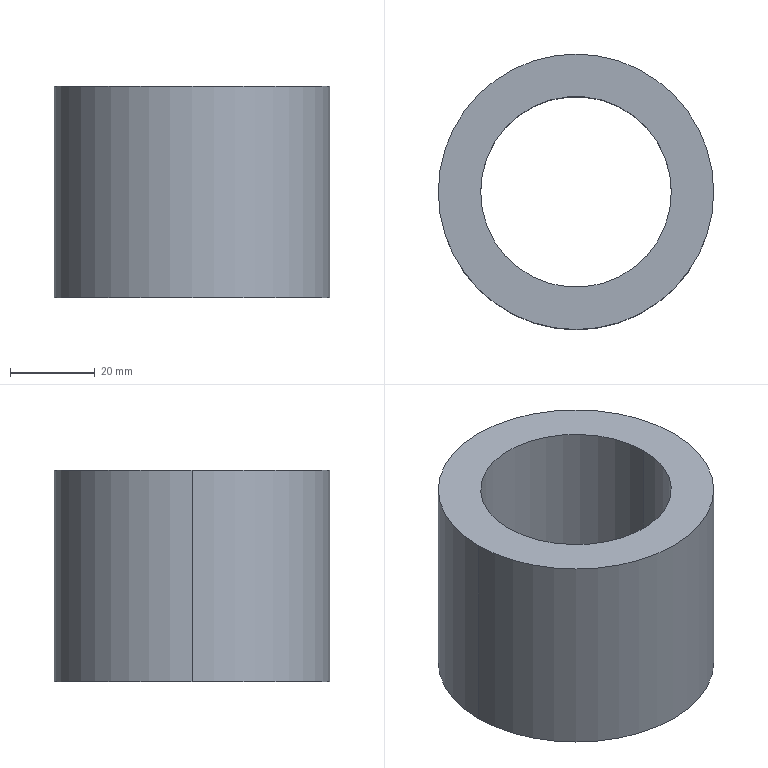Part | SolidWorks | features Extrusion 1 | 1 solid | 6 faces | box 65 x 65 x 50 mm | volume 86394 mm3 | cylinder 4 | plane 2 | commonest cylinder face diameters 45 x2 65 x2
STEP:
#1=CARTESIAN_POINT('',(-22.5,0.,50.));
#2=VERTEX_POINT('',#1);
#3=CARTESIAN_POINT('',(22.5,0.,50.));
#4=VERTEX_POINT('',#3);
#5=CARTESIAN_POINT('',(0.,0.,50.));
#6=DIRECTION('',(0.,0.,1.));
#7=DIRECTION('',(1.,0.,0.));
#8=AXIS2_PLACEMENT_3D('',#5,#6,#7);
#9=CIRCLE('',#8,22.5);
#10=EDGE_CURVE('',#2,#4,#9,.T.);
#11=ORIENTED_EDGE('',*,*,#10,.T.);
#12=CARTESIAN_POINT('',(22.5,0.,0.));
#13=VERTEX_POINT('',#12);
#14=CARTESIAN_POINT('',(22.5,0.,50.));
#15=DIRECTION('',(0.,0.,-1.));
#16=VECTOR('',#15,1000.);
#17=LINE('',#14,#16);
#18=EDGE_CURVE('',#4,#13,#17,.T.);
#19=ORIENTED_EDGE('',*,*,#18,.T.);
#20=CARTESIAN_POINT('',(-22.5,0.,0.));
#21=VERTEX_POINT('',#20);
#22=CARTESIAN_POINT('',(0.,0.,0.));
#23=DIRECTION('',(0.,0.,1.));
#24=DIRECTION('',(1.,0.,0.));
#25=AXIS2_PLACEMENT_3D('',#22,#23,#24);
#26=CIRCLE('',#25,22.5);
#27=EDGE_CURVE('',#21,#13,#26,.T.);
#28=ORIENTED_EDGE('',*,*,#27,.F.);
#29=CARTESIAN_POINT('',(-22.5,0.,50.));
#30=DIRECTION('',(0.,0.,-1.));
#31=VECTOR('',#30,1000.);
#32=LINE('',#29,#31);
#33=EDGE_CURVE('',#2,#21,#32,.T.);
#34=ORIENTED_EDGE('',*,*,#33,.F.);
#35=EDGE_LOOP('',(#11,#19,#28,#34));
#36=FACE_OUTER_BOUND('',#35,.T.);
#37=CARTESIAN_POINT('',(0.,0.,50.));
#38=DIRECTION('',(0.,0.,-1.));
#39=DIRECTION('',(-1.,0.,0.));
#40=AXIS2_PLACEMENT_3D('',#37,#38,#39);
#41=CYLINDRICAL_SURFACE('',#40,22.5);
#42=ADVANCED_FACE('',(#36),#41,.F.);
#43=CARTESIAN_POINT('',(32.5,0.,50.));
#44=VERTEX_POINT('',#43);
#45=CARTESIAN_POINT('',(-32.5,0.,50.));
#46=VERTEX_POINT('',#45);
#47=CARTESIAN_POINT('',(0.,0.,50.));
#48=DIRECTION('',(0.,0.,1.));
#49=DIRECTION('',(1.,0.,0.));
#50=AXIS2_PLACEMENT_3D('',#47,#48,#49);
#51=CIRCLE('',#50,32.5);
#52=EDGE_CURVE('',#44,#46,#51,.T.);
#53=ORIENTED_EDGE('',*,*,#52,.F.);
#54=CARTESIAN_POINT('',(32.5,0.,0.));
#55=VERTEX_POINT('',#54);
#56=CARTESIAN_POINT('',(32.5,0.,50.));
#57=DIRECTION('',(0.,0.,-1.));
#58=VECTOR('',#57,1000.);
#59=LINE('',#56,#58);
#60=EDGE_CURVE('',#44,#55,#59,.T.);
#61=ORIENTED_EDGE('',*,*,#60,.T.);
#62=CARTESIAN_POINT('',(-32.5,0.,0.));
#63=VERTEX_POINT('',#62);
#64=CARTESIAN_POINT('',(0.,0.,0.));
#65=DIRECTION('',(0.,0.,1.));
#66=DIRECTION('',(1.,0.,0.));
#67=AXIS2_PLACEMENT_3D('',#64,#65,#66);
#68=CIRCLE('',#67,32.5);
#69=EDGE_CURVE('',#55,#63,#68,.T.);
#70=ORIENTED_EDGE('',*,*,#69,.T.);
#71=CARTESIAN_POINT('',(-32.5,0.,50.));
#72=DIRECTION('',(0.,0.,-1.));
#73=VECTOR('',#72,1000.);
#74=LINE('',#71,#73);
#75=EDGE_CURVE('',#46,#63,#74,.T.);
#76=ORIENTED_EDGE('',*,*,#75,.F.);
#77=EDGE_LOOP('',(#53,#61,#70,#76));
#78=FACE_OUTER_BOUND('',#77,.T.);
#79=CARTESIAN_POINT('',(0.,0.,50.));
#80=DIRECTION('',(0.,0.,-1.));
#81=DIRECTION('',(-1.,0.,0.));
#82=AXIS2_PLACEMENT_3D('',#79,#80,#81);
#83=CYLINDRICAL_SURFACE('',#82,32.5);
#84=ADVANCED_FACE('',(#78),#83,.T.);
#85=CARTESIAN_POINT('',(0.,0.,50.));
#86=DIRECTION('',(0.,0.,1.));
#87=DIRECTION('',(1.,0.,0.));
#88=AXIS2_PLACEMENT_3D('',#85,#86,#87);
#89=CIRCLE('',#88,32.5);
#90=EDGE_CURVE('',#46,#44,#89,.T.);
#91=ORIENTED_EDGE('',*,*,#90,.T.);
#92=ORIENTED_EDGE('',*,*,#52,.T.);
#93=EDGE_LOOP('',(#91,#92));
#94=FACE_OUTER_BOUND('',#93,.T.);
#95=ORIENTED_EDGE('',*,*,#10,.F.);
#96=CARTESIAN_POINT('',(0.,0.,50.));
#97=DIRECTION('',(0.,0.,1.));
#98=DIRECTION('',(1.,0.,0.));
#99=AXIS2_PLACEMENT_3D('',#96,#97,#98);
#100=CIRCLE('',#99,22.5);
#101=EDGE_CURVE('',#4,#2,#100,.T.);
#102=ORIENTED_EDGE('',*,*,#101,.F.);
#103=EDGE_LOOP('',(#95,#102));
#104=FACE_BOUND('',#103,.T.);
#105=CARTESIAN_POINT('',(0.,0.,50.));
#106=DIRECTION('',(0.,0.,1.));
#107=DIRECTION('',(1.,0.,0.));
#108=AXIS2_PLACEMENT_3D('',#105,#106,#107);
#109=PLANE('',#108);
#110=ADVANCED_FACE('',(#94,#104),#109,.T.);
#111=CARTESIAN_POINT('',(0.,0.,0.));
#112=DIRECTION('',(0.,0.,1.));
#113=DIRECTION('',(1.,0.,0.));
#114=AXIS2_PLACEMENT_3D('',#111,#112,#113);
#115=CIRCLE('',#114,32.5);
#116=EDGE_CURVE('',#63,#55,#115,.T.);
#117=ORIENTED_EDGE('',*,*,#116,.F.);
#118=ORIENTED_EDGE('',*,*,#69,.F.);
#119=EDGE_LOOP('',(#117,#118));
#120=FACE_OUTER_BOUND('',#119,.T.);
#121=ORIENTED_EDGE('',*,*,#27,.T.);
#122=CARTESIAN_POINT('',(0.,0.,0.));
#123=DIRECTION('',(0.,0.,1.));
#124=DIRECTION('',(1.,0.,0.));
#125=AXIS2_PLACEMENT_3D('',#122,#123,#124);
#126=CIRCLE('',#125,22.5);
#127=EDGE_CURVE('',#13,#21,#126,.T.);
#128=ORIENTED_EDGE('',*,*,#127,.T.);
#129=EDGE_LOOP('',(#121,#128));
#130=FACE_BOUND('',#129,.T.);
#131=CARTESIAN_POINT('',(0.,0.,0.));
#132=DIRECTION('',(0.,0.,1.));
#133=DIRECTION('',(1.,0.,0.));
#134=AXIS2_PLACEMENT_3D('',#131,#132,#133);
#135=PLANE('',#134);
#136=ADVANCED_FACE('',(#120,#130),#135,.F.);
#137=ORIENTED_EDGE('',*,*,#60,.F.);
#138=ORIENTED_EDGE('',*,*,#90,.F.);
#139=ORIENTED_EDGE('',*,*,#75,.T.);
#140=ORIENTED_EDGE('',*,*,#116,.T.);
#141=EDGE_LOOP('',(#137,#138,#139,#140));
#142=FACE_OUTER_BOUND('',#141,.T.);
#143=CARTESIAN_POINT('',(0.,0.,50.));
#144=DIRECTION('',(0.,0.,-1.));
#145=DIRECTION('',(-1.,0.,0.));
#146=AXIS2_PLACEMENT_3D('',#143,#144,#145);
#147=CYLINDRICAL_SURFACE('',#146,32.5);
#148=ADVANCED_FACE('',(#142),#147,.T.);
#149=ORIENTED_EDGE('',*,*,#18,.F.);
#150=ORIENTED_EDGE('',*,*,#101,.T.);
#151=ORIENTED_EDGE('',*,*,#33,.T.);
#152=ORIENTED_EDGE('',*,*,#127,.F.);
#153=EDGE_LOOP('',(#149,#150,#151,#152));
#154=FACE_OUTER_BOUND('',#153,.T.);
#155=CARTESIAN_POINT('',(0.,0.,50.));
#156=DIRECTION('',(0.,0.,-1.));
#157=DIRECTION('',(-1.,0.,0.));
#158=AXIS2_PLACEMENT_3D('',#155,#156,#157);
#159=CYLINDRICAL_SURFACE('',#158,22.5);
#160=ADVANCED_FACE('',(#154),#159,.F.);
#161=CLOSED_SHELL('',(#42,#84,#110,#136,#148,#160));
#162=MANIFOLD_SOLID_BREP('',#161);
#163=CARTESIAN_POINT('',(0.,0.,0.));
#164=DIRECTION('',(0.,0.,1.));
#165=DIRECTION('',(1.,0.,0.));
#166=AXIS2_PLACEMENT_3D('',#163,#164,#165);
#167=(LENGTH_UNIT()NAMED_UNIT(*)SI_UNIT(.MILLI.,.METRE.));
#168=UNCERTAINTY_MEASURE_WITH_UNIT(LENGTH_MEASURE(0.00001),#167,'','');
#169=(NAMED_UNIT(*)PLANE_ANGLE_UNIT()SI_UNIT($,.RADIAN.));
#170=(NAMED_UNIT(*)SI_UNIT($,.STERADIAN.)SOLID_ANGLE_UNIT());
#171=(GEOMETRIC_REPRESENTATION_CONTEXT(3)GLOBAL_UNCERTAINTY_ASSIGNED_CONTEXT((#168))GLOBAL_UNIT_ASSIGNED_CONTEXT((#167,#169,#170))REPRESENTATION_CONTEXT('',''));
#172=ADVANCED_BREP_SHAPE_REPRESENTATION('',(#162,#166),#171);